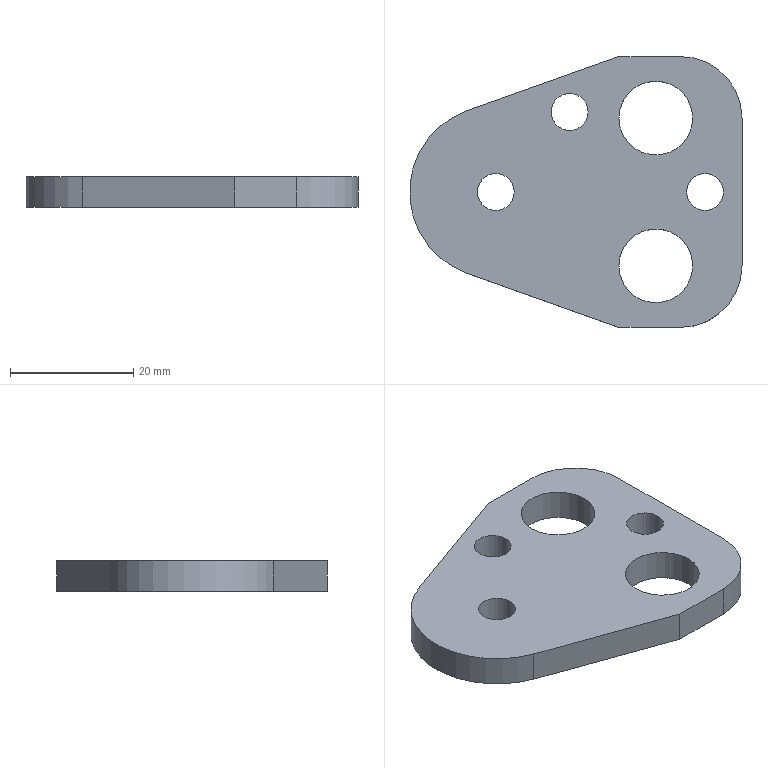Part | NX | features solid 2 | 1 solid | 15 faces | box 54 x 44 x 5 mm | volume 7870 mm3 | cylinder 8 | plane 7 | commonest cylinder face diameters 6 x3 12 x2 20 x2 28 x1
STEP:
#1=CARTESIAN_POINT('',(-689.702,-197.243,110.));
#2=VERTEX_POINT('',#1);
#3=CARTESIAN_POINT('',(-664.997,-206.057,110.));
#4=VERTEX_POINT('',#3);
#5=CARTESIAN_POINT('',(-689.702,-197.243,110.));
#6=DIRECTION('',(0.9418,-0.336,0.));
#7=VECTOR('',#6,1000.);
#8=LINE('',#5,#7);
#9=EDGE_CURVE('',#2,#4,#8,.T.);
#10=ORIENTED_EDGE('',*,*,#9,.F.);
#11=CARTESIAN_POINT('',(-689.702,-197.243,105.));
#12=VERTEX_POINT('',#11);
#13=CARTESIAN_POINT('',(-689.702,-197.243,105.));
#14=DIRECTION('',(0.,0.,1.));
#15=VECTOR('',#14,1000.);
#16=LINE('',#13,#15);
#17=EDGE_CURVE('',#12,#2,#16,.T.);
#18=ORIENTED_EDGE('',*,*,#17,.F.);
#19=CARTESIAN_POINT('',(-664.997,-206.057,105.));
#20=VERTEX_POINT('',#19);
#21=CARTESIAN_POINT('',(-689.702,-197.243,105.));
#22=DIRECTION('',(0.9418,-0.336,0.));
#23=VECTOR('',#22,1000.);
#24=LINE('',#21,#23);
#25=EDGE_CURVE('',#12,#20,#24,.T.);
#26=ORIENTED_EDGE('',*,*,#25,.T.);
#27=CARTESIAN_POINT('',(-664.997,-206.057,105.));
#28=DIRECTION('',(0.,0.,1.));
#29=VECTOR('',#28,1000.);
#30=LINE('',#27,#29);
#31=EDGE_CURVE('',#20,#4,#30,.T.);
#32=ORIENTED_EDGE('',*,*,#31,.T.);
#33=EDGE_LOOP('',(#10,#18,#26,#32));
#34=FACE_BOUND('',#33,.T.);
#35=CARTESIAN_POINT('',(-689.702,-197.243,105.));
#36=DIRECTION('',(-0.336,-0.9418,0.));
#37=DIRECTION('',(0.9418,-0.336,0.));
#38=AXIS2_PLACEMENT_3D('',#35,#36,#37);
#39=PLANE('',#38);
#40=ADVANCED_FACE('',(#34),#39,.T.);
#41=CARTESIAN_POINT('',(-654.997,-206.057,110.));
#42=VERTEX_POINT('',#41);
#43=CARTESIAN_POINT('',(-664.997,-206.057,110.));
#44=DIRECTION('',(1.,0.,0.));
#45=VECTOR('',#44,1000.);
#46=LINE('',#43,#45);
#47=EDGE_CURVE('',#4,#42,#46,.T.);
#48=ORIENTED_EDGE('',*,*,#47,.F.);
#49=ORIENTED_EDGE('',*,*,#31,.F.);
#50=CARTESIAN_POINT('',(-654.997,-206.057,105.));
#51=VERTEX_POINT('',#50);
#52=CARTESIAN_POINT('',(-664.997,-206.057,105.));
#53=DIRECTION('',(1.,0.,0.));
#54=VECTOR('',#53,1000.);
#55=LINE('',#52,#54);
#56=EDGE_CURVE('',#20,#51,#55,.T.);
#57=ORIENTED_EDGE('',*,*,#56,.T.);
#58=CARTESIAN_POINT('',(-654.997,-206.057,105.));
#59=DIRECTION('',(0.,0.,1.));
#60=VECTOR('',#59,1000.);
#61=LINE('',#58,#60);
#62=EDGE_CURVE('',#51,#42,#61,.T.);
#63=ORIENTED_EDGE('',*,*,#62,.T.);
#64=EDGE_LOOP('',(#48,#49,#57,#63));
#65=FACE_BOUND('',#64,.T.);
#66=CARTESIAN_POINT('',(-664.997,-206.057,105.));
#67=DIRECTION('',(0.,-1.,0.));
#68=DIRECTION('',(0.,0.,1.));
#69=AXIS2_PLACEMENT_3D('',#66,#67,#68);
#70=PLANE('',#69);
#71=ADVANCED_FACE('',(#65),#70,.T.);
#72=CARTESIAN_POINT('',(-644.997,-196.057,110.));
#73=VERTEX_POINT('',#72);
#74=CARTESIAN_POINT('',(-654.997,-196.057,110.));
#75=DIRECTION('',(0.,0.,-1.));
#76=DIRECTION('',(1.,0.,0.));
#77=AXIS2_PLACEMENT_3D('',#74,#75,#76);
#78=CIRCLE('',#77,10.);
#79=EDGE_CURVE('',#73,#42,#78,.T.);
#80=ORIENTED_EDGE('',*,*,#79,.T.);
#81=ORIENTED_EDGE('',*,*,#62,.F.);
#82=CARTESIAN_POINT('',(-644.997,-196.057,105.));
#83=VERTEX_POINT('',#82);
#84=CARTESIAN_POINT('',(-654.997,-196.057,105.));
#85=DIRECTION('',(0.,0.,-1.));
#86=DIRECTION('',(1.,0.,0.));
#87=AXIS2_PLACEMENT_3D('',#84,#85,#86);
#88=CIRCLE('',#87,10.);
#89=EDGE_CURVE('',#83,#51,#88,.T.);
#90=ORIENTED_EDGE('',*,*,#89,.F.);
#91=CARTESIAN_POINT('',(-644.997,-196.057,105.));
#92=DIRECTION('',(0.,0.,1.));
#93=VECTOR('',#92,1000.);
#94=LINE('',#91,#93);
#95=EDGE_CURVE('',#83,#73,#94,.T.);
#96=ORIENTED_EDGE('',*,*,#95,.T.);
#97=EDGE_LOOP('',(#80,#81,#90,#96));
#98=FACE_BOUND('',#97,.T.);
#99=CARTESIAN_POINT('',(-654.997,-196.057,105.));
#100=DIRECTION('',(0.,0.,1.));
#101=DIRECTION('',(-1.,0.,0.));
#102=AXIS2_PLACEMENT_3D('',#99,#100,#101);
#103=CYLINDRICAL_SURFACE('',#102,10.);
#104=ADVANCED_FACE('',(#98),#103,.T.);
#105=CARTESIAN_POINT('',(-644.997,-172.057,110.));
#106=VERTEX_POINT('',#105);
#107=CARTESIAN_POINT('',(-644.997,-196.057,110.));
#108=DIRECTION('',(0.,1.,0.));
#109=VECTOR('',#108,1000.);
#110=LINE('',#107,#109);
#111=EDGE_CURVE('',#73,#106,#110,.T.);
#112=ORIENTED_EDGE('',*,*,#111,.F.);
#113=ORIENTED_EDGE('',*,*,#95,.F.);
#114=CARTESIAN_POINT('',(-644.997,-172.057,105.));
#115=VERTEX_POINT('',#114);
#116=CARTESIAN_POINT('',(-644.997,-196.057,105.));
#117=DIRECTION('',(0.,1.,0.));
#118=VECTOR('',#117,1000.);
#119=LINE('',#116,#118);
#120=EDGE_CURVE('',#83,#115,#119,.T.);
#121=ORIENTED_EDGE('',*,*,#120,.T.);
#122=CARTESIAN_POINT('',(-644.997,-172.057,105.));
#123=DIRECTION('',(0.,0.,1.));
#124=VECTOR('',#123,1000.);
#125=LINE('',#122,#124);
#126=EDGE_CURVE('',#115,#106,#125,.T.);
#127=ORIENTED_EDGE('',*,*,#126,.T.);
#128=EDGE_LOOP('',(#112,#113,#121,#127));
#129=FACE_BOUND('',#128,.T.);
#130=CARTESIAN_POINT('',(-644.997,-196.057,105.));
#131=DIRECTION('',(1.,0.,0.));
#132=DIRECTION('',(0.,1.,0.));
#133=AXIS2_PLACEMENT_3D('',#130,#131,#132);
#134=PLANE('',#133);
#135=ADVANCED_FACE('',(#129),#134,.T.);
#136=CARTESIAN_POINT('',(-654.997,-162.057,110.));
#137=VERTEX_POINT('',#136);
#138=CARTESIAN_POINT('',(-654.997,-172.057,110.));
#139=DIRECTION('',(0.,0.,-1.));
#140=DIRECTION('',(1.,0.,0.));
#141=AXIS2_PLACEMENT_3D('',#138,#139,#140);
#142=CIRCLE('',#141,10.);
#143=EDGE_CURVE('',#137,#106,#142,.T.);
#144=ORIENTED_EDGE('',*,*,#143,.T.);
#145=ORIENTED_EDGE('',*,*,#126,.F.);
#146=CARTESIAN_POINT('',(-654.997,-162.057,105.));
#147=VERTEX_POINT('',#146);
#148=CARTESIAN_POINT('',(-654.997,-172.057,105.));
#149=DIRECTION('',(0.,0.,-1.));
#150=DIRECTION('',(1.,0.,0.));
#151=AXIS2_PLACEMENT_3D('',#148,#149,#150);
#152=CIRCLE('',#151,10.);
#153=EDGE_CURVE('',#147,#115,#152,.T.);
#154=ORIENTED_EDGE('',*,*,#153,.F.);
#155=CARTESIAN_POINT('',(-654.997,-162.057,105.));
#156=DIRECTION('',(0.,0.,1.));
#157=VECTOR('',#156,1000.);
#158=LINE('',#155,#157);
#159=EDGE_CURVE('',#147,#137,#158,.T.);
#160=ORIENTED_EDGE('',*,*,#159,.T.);
#161=EDGE_LOOP('',(#144,#145,#154,#160));
#162=FACE_BOUND('',#161,.T.);
#163=CARTESIAN_POINT('',(-654.997,-172.057,105.));
#164=DIRECTION('',(0.,0.,1.));
#165=DIRECTION('',(-1.,0.,0.));
#166=AXIS2_PLACEMENT_3D('',#163,#164,#165);
#167=CYLINDRICAL_SURFACE('',#166,10.);
#168=ADVANCED_FACE('',(#162),#167,.T.);
#169=CARTESIAN_POINT('',(-664.997,-162.057,110.));
#170=VERTEX_POINT('',#169);
#171=CARTESIAN_POINT('',(-664.997,-162.057,110.));
#172=DIRECTION('',(1.,0.,0.));
#173=VECTOR('',#172,1000.);
#174=LINE('',#171,#173);
#175=EDGE_CURVE('',#170,#137,#174,.T.);
#176=ORIENTED_EDGE('',*,*,#175,.T.);
#177=ORIENTED_EDGE('',*,*,#159,.F.);
#178=CARTESIAN_POINT('',(-664.997,-162.057,105.));
#179=VERTEX_POINT('',#178);
#180=CARTESIAN_POINT('',(-664.997,-162.057,105.));
#181=DIRECTION('',(1.,0.,0.));
#182=VECTOR('',#181,1000.);
#183=LINE('',#180,#182);
#184=EDGE_CURVE('',#179,#147,#183,.T.);
#185=ORIENTED_EDGE('',*,*,#184,.F.);
#186=CARTESIAN_POINT('',(-664.997,-162.057,105.));
#187=DIRECTION('',(0.,0.,1.));
#188=VECTOR('',#187,1000.);
#189=LINE('',#186,#188);
#190=EDGE_CURVE('',#179,#170,#189,.T.);
#191=ORIENTED_EDGE('',*,*,#190,.T.);
#192=EDGE_LOOP('',(#176,#177,#185,#191));
#193=FACE_BOUND('',#192,.T.);
#194=CARTESIAN_POINT('',(-664.997,-162.057,105.));
#195=DIRECTION('',(0.,-1.,0.));
#196=DIRECTION('',(1.,0.,0.));
#197=AXIS2_PLACEMENT_3D('',#194,#195,#196);
#198=PLANE('',#197);
#199=ADVANCED_FACE('',(#193),#198,.F.);
#200=CARTESIAN_POINT('',(-689.702,-170.871,110.));
#201=VERTEX_POINT('',#200);
#202=CARTESIAN_POINT('',(-689.702,-170.871,110.));
#203=DIRECTION('',(0.9418,0.336,0.));
#204=VECTOR('',#203,1000.);
#205=LINE('',#202,#204);
#206=EDGE_CURVE('',#201,#170,#205,.T.);
#207=ORIENTED_EDGE('',*,*,#206,.T.);
#208=ORIENTED_EDGE('',*,*,#190,.F.);
#209=CARTESIAN_POINT('',(-689.702,-170.871,105.));
#210=VERTEX_POINT('',#209);
#211=CARTESIAN_POINT('',(-689.702,-170.871,105.));
#212=DIRECTION('',(0.9418,0.336,0.));
#213=VECTOR('',#212,1000.);
#214=LINE('',#211,#213);
#215=EDGE_CURVE('',#210,#179,#214,.T.);
#216=ORIENTED_EDGE('',*,*,#215,.F.);
#217=CARTESIAN_POINT('',(-689.702,-170.871,105.));
#218=DIRECTION('',(0.,0.,1.));
#219=VECTOR('',#218,1000.);
#220=LINE('',#217,#219);
#221=EDGE_CURVE('',#210,#201,#220,.T.);
#222=ORIENTED_EDGE('',*,*,#221,.T.);
#223=EDGE_LOOP('',(#207,#208,#216,#222));
#224=FACE_BOUND('',#223,.T.);
#225=CARTESIAN_POINT('',(-689.702,-170.871,105.));
#226=DIRECTION('',(0.336,-0.9418,0.));
#227=DIRECTION('',(0.9418,0.336,0.));
#228=AXIS2_PLACEMENT_3D('',#225,#226,#227);
#229=PLANE('',#228);
#230=ADVANCED_FACE('',(#224),#229,.F.);
#231=CARTESIAN_POINT('',(-652.997,-196.057,105.));
#232=VERTEX_POINT('',#231);
#233=CARTESIAN_POINT('',(-658.997,-196.057,105.));
#234=DIRECTION('',(0.,0.,-1.));
#235=DIRECTION('',(1.,0.,0.));
#236=AXIS2_PLACEMENT_3D('',#233,#234,#235);
#237=CIRCLE('',#236,6.);
#238=EDGE_CURVE('',#232,#232,#237,.T.);
#239=ORIENTED_EDGE('',*,*,#238,.T.);
#240=EDGE_LOOP('',(#239));
#241=FACE_BOUND('',#240,.T.);
#242=CARTESIAN_POINT('',(-652.997,-196.057,110.));
#243=VERTEX_POINT('',#242);
#244=CARTESIAN_POINT('',(-658.997,-196.057,110.));
#245=DIRECTION('',(0.,0.,-1.));
#246=DIRECTION('',(1.,0.,0.));
#247=AXIS2_PLACEMENT_3D('',#244,#245,#246);
#248=CIRCLE('',#247,6.);
#249=EDGE_CURVE('',#243,#243,#248,.T.);
#250=ORIENTED_EDGE('',*,*,#249,.F.);
#251=EDGE_LOOP('',(#250));
#252=FACE_BOUND('',#251,.T.);
#253=CARTESIAN_POINT('',(-658.997,-196.057,105.));
#254=DIRECTION('',(0.,0.,1.));
#255=DIRECTION('',(-1.,0.,0.));
#256=AXIS2_PLACEMENT_3D('',#253,#254,#255);
#257=CYLINDRICAL_SURFACE('',#256,6.);
#258=ADVANCED_FACE('',(#241,#252),#257,.F.);
#259=CARTESIAN_POINT('',(-681.997,-184.057,105.));
#260=VERTEX_POINT('',#259);
#261=CARTESIAN_POINT('',(-684.997,-184.057,105.));
#262=DIRECTION('',(0.,0.,-1.));
#263=DIRECTION('',(1.,0.,0.));
#264=AXIS2_PLACEMENT_3D('',#261,#262,#263);
#265=CIRCLE('',#264,3.);
#266=EDGE_CURVE('',#260,#260,#265,.T.);
#267=ORIENTED_EDGE('',*,*,#266,.T.);
#268=EDGE_LOOP('',(#267));
#269=FACE_BOUND('',#268,.T.);
#270=CARTESIAN_POINT('',(-681.997,-184.057,110.));
#271=VERTEX_POINT('',#270);
#272=CARTESIAN_POINT('',(-684.997,-184.057,110.));
#273=DIRECTION('',(0.,0.,-1.));
#274=DIRECTION('',(1.,0.,0.));
#275=AXIS2_PLACEMENT_3D('',#272,#273,#274);
#276=CIRCLE('',#275,3.);
#277=EDGE_CURVE('',#271,#271,#276,.T.);
#278=ORIENTED_EDGE('',*,*,#277,.F.);
#279=EDGE_LOOP('',(#278));
#280=FACE_BOUND('',#279,.T.);
#281=CARTESIAN_POINT('',(-684.997,-184.057,105.));
#282=DIRECTION('',(0.,0.,-1.));
#283=DIRECTION('',(1.,0.,0.));
#284=AXIS2_PLACEMENT_3D('',#281,#282,#283);
#285=CYLINDRICAL_SURFACE('',#284,3.);
#286=ADVANCED_FACE('',(#269,#280),#285,.F.);
#287=CARTESIAN_POINT('',(-684.997,-184.057,110.));
#288=DIRECTION('',(0.,0.,-1.));
#289=DIRECTION('',(1.,0.,0.));
#290=AXIS2_PLACEMENT_3D('',#287,#288,#289);
#291=CIRCLE('',#290,14.);
#292=EDGE_CURVE('',#2,#201,#291,.T.);
#293=ORIENTED_EDGE('',*,*,#292,.T.);
#294=ORIENTED_EDGE('',*,*,#221,.F.);
#295=CARTESIAN_POINT('',(-684.997,-184.057,105.));
#296=DIRECTION('',(0.,0.,-1.));
#297=DIRECTION('',(1.,0.,0.));
#298=AXIS2_PLACEMENT_3D('',#295,#296,#297);
#299=CIRCLE('',#298,14.);
#300=EDGE_CURVE('',#12,#210,#299,.T.);
#301=ORIENTED_EDGE('',*,*,#300,.F.);
#302=ORIENTED_EDGE('',*,*,#17,.T.);
#303=EDGE_LOOP('',(#293,#294,#301,#302));
#304=FACE_BOUND('',#303,.T.);
#305=CARTESIAN_POINT('',(-684.997,-184.057,105.));
#306=DIRECTION('',(0.,0.,1.));
#307=DIRECTION('',(-1.,0.,0.));
#308=AXIS2_PLACEMENT_3D('',#305,#306,#307);
#309=CYLINDRICAL_SURFACE('',#308,14.);
#310=ADVANCED_FACE('',(#304),#309,.T.);
#311=CARTESIAN_POINT('',(-652.997,-172.057,105.));
#312=VERTEX_POINT('',#311);
#313=CARTESIAN_POINT('',(-658.997,-172.057,105.));
#314=DIRECTION('',(0.,0.,-1.));
#315=DIRECTION('',(1.,0.,0.));
#316=AXIS2_PLACEMENT_3D('',#313,#314,#315);
#317=CIRCLE('',#316,6.);
#318=EDGE_CURVE('',#312,#312,#317,.T.);
#319=ORIENTED_EDGE('',*,*,#318,.T.);
#320=EDGE_LOOP('',(#319));
#321=FACE_BOUND('',#320,.T.);
#322=CARTESIAN_POINT('',(-652.997,-172.057,110.));
#323=VERTEX_POINT('',#322);
#324=CARTESIAN_POINT('',(-658.997,-172.057,110.));
#325=DIRECTION('',(0.,0.,-1.));
#326=DIRECTION('',(1.,0.,0.));
#327=AXIS2_PLACEMENT_3D('',#324,#325,#326);
#328=CIRCLE('',#327,6.);
#329=EDGE_CURVE('',#323,#323,#328,.T.);
#330=ORIENTED_EDGE('',*,*,#329,.F.);
#331=EDGE_LOOP('',(#330));
#332=FACE_BOUND('',#331,.T.);
#333=CARTESIAN_POINT('',(-658.997,-172.057,105.));
#334=DIRECTION('',(0.,0.,1.));
#335=DIRECTION('',(-1.,0.,0.));
#336=AXIS2_PLACEMENT_3D('',#333,#334,#335);
#337=CYLINDRICAL_SURFACE('',#336,6.);
#338=ADVANCED_FACE('',(#321,#332),#337,.F.);
#339=CARTESIAN_POINT('',(-669.997,-171.057,105.));
#340=VERTEX_POINT('',#339);
#341=CARTESIAN_POINT('',(-672.997,-171.057,105.));
#342=DIRECTION('',(0.,0.,-1.));
#343=DIRECTION('',(1.,0.,0.));
#344=AXIS2_PLACEMENT_3D('',#341,#342,#343);
#345=CIRCLE('',#344,3.);
#346=EDGE_CURVE('',#340,#340,#345,.T.);
#347=ORIENTED_EDGE('',*,*,#346,.T.);
#348=EDGE_LOOP('',(#347));
#349=FACE_BOUND('',#348,.T.);
#350=CARTESIAN_POINT('',(-669.997,-171.057,110.));
#351=VERTEX_POINT('',#350);
#352=CARTESIAN_POINT('',(-672.997,-171.057,110.));
#353=DIRECTION('',(0.,0.,-1.));
#354=DIRECTION('',(1.,0.,0.));
#355=AXIS2_PLACEMENT_3D('',#352,#353,#354);
#356=CIRCLE('',#355,3.);
#357=EDGE_CURVE('',#351,#351,#356,.T.);
#358=ORIENTED_EDGE('',*,*,#357,.F.);
#359=EDGE_LOOP('',(#358));
#360=FACE_BOUND('',#359,.T.);
#361=CARTESIAN_POINT('',(-672.997,-171.057,105.));
#362=DIRECTION('',(0.,0.,1.));
#363=DIRECTION('',(-1.,0.,0.));
#364=AXIS2_PLACEMENT_3D('',#361,#362,#363);
#365=CYLINDRICAL_SURFACE('',#364,3.);
#366=ADVANCED_FACE('',(#349,#360),#365,.F.);
#367=CARTESIAN_POINT('',(-647.997,-184.057,105.));
#368=VERTEX_POINT('',#367);
#369=CARTESIAN_POINT('',(-650.997,-184.057,105.));
#370=DIRECTION('',(0.,0.,-1.));
#371=DIRECTION('',(1.,0.,0.));
#372=AXIS2_PLACEMENT_3D('',#369,#370,#371);
#373=CIRCLE('',#372,3.);
#374=EDGE_CURVE('',#368,#368,#373,.T.);
#375=ORIENTED_EDGE('',*,*,#374,.T.);
#376=EDGE_LOOP('',(#375));
#377=FACE_BOUND('',#376,.T.);
#378=CARTESIAN_POINT('',(-647.997,-184.057,110.));
#379=VERTEX_POINT('',#378);
#380=CARTESIAN_POINT('',(-650.997,-184.057,110.));
#381=DIRECTION('',(0.,0.,-1.));
#382=DIRECTION('',(1.,0.,0.));
#383=AXIS2_PLACEMENT_3D('',#380,#381,#382);
#384=CIRCLE('',#383,3.);
#385=EDGE_CURVE('',#379,#379,#384,.T.);
#386=ORIENTED_EDGE('',*,*,#385,.F.);
#387=EDGE_LOOP('',(#386));
#388=FACE_BOUND('',#387,.T.);
#389=CARTESIAN_POINT('',(-650.997,-184.057,105.));
#390=DIRECTION('',(0.,0.,1.));
#391=DIRECTION('',(-1.,0.,0.));
#392=AXIS2_PLACEMENT_3D('',#389,#390,#391);
#393=CYLINDRICAL_SURFACE('',#392,3.);
#394=ADVANCED_FACE('',(#377,#388),#393,.F.);
#395=ORIENTED_EDGE('',*,*,#346,.F.);
#396=EDGE_LOOP('',(#395));
#397=FACE_BOUND('',#396,.T.);
#398=ORIENTED_EDGE('',*,*,#318,.F.);
#399=EDGE_LOOP('',(#398));
#400=FACE_BOUND('',#399,.T.);
#401=ORIENTED_EDGE('',*,*,#25,.F.);
#402=ORIENTED_EDGE('',*,*,#300,.T.);
#403=ORIENTED_EDGE('',*,*,#215,.T.);
#404=ORIENTED_EDGE('',*,*,#184,.T.);
#405=ORIENTED_EDGE('',*,*,#153,.T.);
#406=ORIENTED_EDGE('',*,*,#120,.F.);
#407=ORIENTED_EDGE('',*,*,#89,.T.);
#408=ORIENTED_EDGE('',*,*,#56,.F.);
#409=EDGE_LOOP('',(#401,#402,#403,#404,#405,#406,#407,#408));
#410=FACE_BOUND('',#409,.T.);
#411=ORIENTED_EDGE('',*,*,#266,.F.);
#412=EDGE_LOOP('',(#411));
#413=FACE_BOUND('',#412,.T.);
#414=ORIENTED_EDGE('',*,*,#238,.F.);
#415=EDGE_LOOP('',(#414));
#416=FACE_BOUND('',#415,.T.);
#417=ORIENTED_EDGE('',*,*,#374,.F.);
#418=EDGE_LOOP('',(#417));
#419=FACE_BOUND('',#418,.T.);
#420=CARTESIAN_POINT('',(-654.997,-196.057,105.));
#421=DIRECTION('',(0.,0.,-1.));
#422=DIRECTION('',(1.,0.,0.));
#423=AXIS2_PLACEMENT_3D('',#420,#421,#422);
#424=PLANE('',#423);
#425=ADVANCED_FACE('',(#397,#400,#410,#413,#416,#419),#424,.T.);
#426=ORIENTED_EDGE('',*,*,#357,.T.);
#427=EDGE_LOOP('',(#426));
#428=FACE_BOUND('',#427,.T.);
#429=ORIENTED_EDGE('',*,*,#329,.T.);
#430=EDGE_LOOP('',(#429));
#431=FACE_BOUND('',#430,.T.);
#432=ORIENTED_EDGE('',*,*,#9,.T.);
#433=ORIENTED_EDGE('',*,*,#47,.T.);
#434=ORIENTED_EDGE('',*,*,#79,.F.);
#435=ORIENTED_EDGE('',*,*,#111,.T.);
#436=ORIENTED_EDGE('',*,*,#143,.F.);
#437=ORIENTED_EDGE('',*,*,#175,.F.);
#438=ORIENTED_EDGE('',*,*,#206,.F.);
#439=ORIENTED_EDGE('',*,*,#292,.F.);
#440=EDGE_LOOP('',(#432,#433,#434,#435,#436,#437,#438,#439));
#441=FACE_BOUND('',#440,.T.);
#442=ORIENTED_EDGE('',*,*,#277,.T.);
#443=EDGE_LOOP('',(#442));
#444=FACE_BOUND('',#443,.T.);
#445=ORIENTED_EDGE('',*,*,#249,.T.);
#446=EDGE_LOOP('',(#445));
#447=FACE_BOUND('',#446,.T.);
#448=ORIENTED_EDGE('',*,*,#385,.T.);
#449=EDGE_LOOP('',(#448));
#450=FACE_BOUND('',#449,.T.);
#451=CARTESIAN_POINT('',(-654.997,-196.057,110.));
#452=DIRECTION('',(0.,0.,-1.));
#453=DIRECTION('',(1.,0.,0.));
#454=AXIS2_PLACEMENT_3D('',#451,#452,#453);
#455=PLANE('',#454);
#456=ADVANCED_FACE('',(#428,#431,#441,#444,#447,#450),#455,.F.);
#457=CLOSED_SHELL('',(#40,#71,#104,#135,#168,#199,#230,#258,#286,#310,#338,#366,#394,#425,#456));
#458=MANIFOLD_SOLID_BREP('',#457);
#459=(LENGTH_UNIT()NAMED_UNIT(*)SI_UNIT(.MILLI.,.METRE.));
#460=UNCERTAINTY_MEASURE_WITH_UNIT(LENGTH_MEASURE(0.00001),#459,'','');
#461=(NAMED_UNIT(*)PLANE_ANGLE_UNIT()SI_UNIT($,.RADIAN.));
#462=(NAMED_UNIT(*)SI_UNIT($,.STERADIAN.)SOLID_ANGLE_UNIT());
#463=(GEOMETRIC_REPRESENTATION_CONTEXT(3)GLOBAL_UNCERTAINTY_ASSIGNED_CONTEXT((#460))GLOBAL_UNIT_ASSIGNED_CONTEXT((#459,#461,#462))REPRESENTATION_CONTEXT('',''));
#464=ADVANCED_BREP_SHAPE_REPRESENTATION('',(#458),#463);